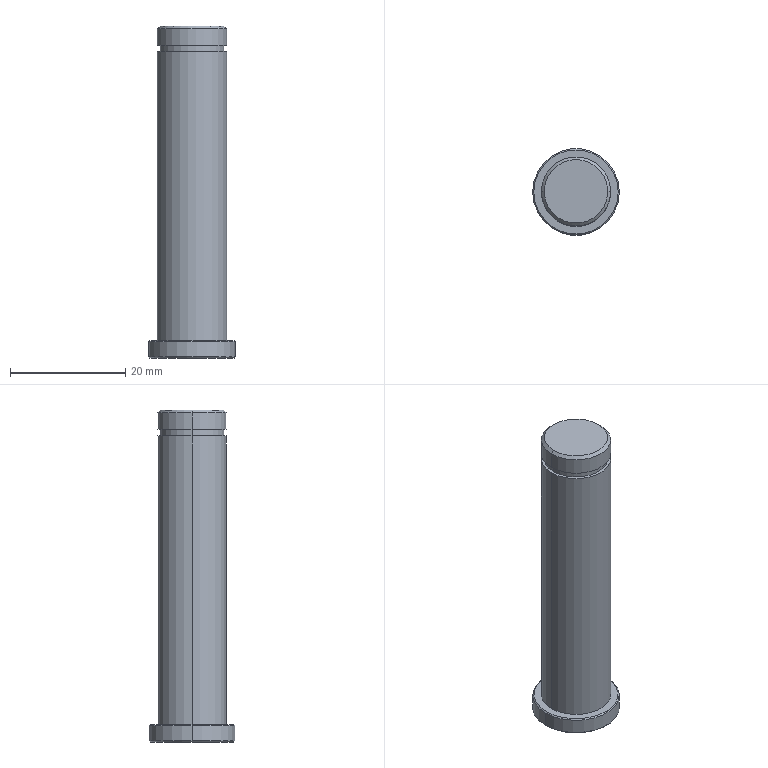Part | SolidWorks | features Chamfer 2, Extrusion 1, ICE 1, RefAxis 1, RevCut 1 | 1 solid | 19 faces | box 15 x 15 x 57.5 mm | volume 6667 mm3 | cylinder 8 | cone 6 | plane 5 | commonest cylinder face diameters 12 x4 11 x2 15 x2
STEP:
#1=CARTESIAN_POINT('',(5.5,0.,57.5));
#2=VERTEX_POINT('',#1);
#3=CARTESIAN_POINT('',(-5.5,0.,57.5));
#4=VERTEX_POINT('',#3);
#5=CARTESIAN_POINT('',(0.,0.,57.5));
#6=DIRECTION('',(0.,0.,1.));
#7=DIRECTION('',(1.,0.,0.));
#8=AXIS2_PLACEMENT_3D('',#5,#6,#7);
#9=CIRCLE('',#8,5.5);
#10=EDGE_CURVE('',#2,#4,#9,.T.);
#11=ORIENTED_EDGE('',*,*,#10,.F.);
#12=CARTESIAN_POINT('',(6.,0.,57.));
#13=VERTEX_POINT('',#12);
#14=CARTESIAN_POINT('',(5.5,0.,57.5));
#15=DIRECTION('',(0.7071,0.,-0.7071));
#16=VECTOR('',#15,1000.);
#17=LINE('',#14,#16);
#18=EDGE_CURVE('',#2,#13,#17,.T.);
#19=ORIENTED_EDGE('',*,*,#18,.T.);
#20=CARTESIAN_POINT('',(-6.,0.,57.));
#21=VERTEX_POINT('',#20);
#22=CARTESIAN_POINT('',(0.,0.,57.));
#23=DIRECTION('',(0.,0.,-1.));
#24=DIRECTION('',(1.,0.,0.));
#25=AXIS2_PLACEMENT_3D('',#22,#23,#24);
#26=CIRCLE('',#25,6.);
#27=EDGE_CURVE('',#21,#13,#26,.T.);
#28=ORIENTED_EDGE('',*,*,#27,.F.);
#29=CARTESIAN_POINT('',(-5.5,0.,57.5));
#30=DIRECTION('',(-0.7071,0.,-0.7071));
#31=VECTOR('',#30,1000.);
#32=LINE('',#29,#31);
#33=EDGE_CURVE('',#4,#21,#32,.T.);
#34=ORIENTED_EDGE('',*,*,#33,.F.);
#35=EDGE_LOOP('',(#11,#19,#28,#34));
#36=FACE_OUTER_BOUND('',#35,.T.);
#37=CARTESIAN_POINT('',(0.,0.,57.5));
#38=DIRECTION('',(0.,0.,-1.));
#39=DIRECTION('',(-1.,0.,0.));
#40=AXIS2_PLACEMENT_3D('',#37,#38,#39);
#41=CONICAL_SURFACE('',#40,5.5,0.7854);
#42=ADVANCED_FACE('',(#36),#41,.T.);
#43=ORIENTED_EDGE('',*,*,#27,.T.);
#44=CARTESIAN_POINT('',(6.,0.,54.15));
#45=VERTEX_POINT('',#44);
#46=CARTESIAN_POINT('',(6.,0.,57.5));
#47=DIRECTION('',(0.,0.,-1.));
#48=VECTOR('',#47,1000.);
#49=LINE('',#46,#48);
#50=EDGE_CURVE('',#13,#45,#49,.T.);
#51=ORIENTED_EDGE('',*,*,#50,.T.);
#52=CARTESIAN_POINT('',(-6.,0.,54.15));
#53=VERTEX_POINT('',#52);
#54=CARTESIAN_POINT('',(0.,0.,54.15));
#55=DIRECTION('',(0.,0.,1.));
#56=DIRECTION('',(1.,0.,0.));
#57=AXIS2_PLACEMENT_3D('',#54,#55,#56);
#58=CIRCLE('',#57,6.);
#59=EDGE_CURVE('',#45,#53,#58,.T.);
#60=ORIENTED_EDGE('',*,*,#59,.T.);
#61=CARTESIAN_POINT('',(-6.,0.,57.5));
#62=DIRECTION('',(0.,0.,-1.));
#63=VECTOR('',#62,1000.);
#64=LINE('',#61,#63);
#65=EDGE_CURVE('',#21,#53,#64,.T.);
#66=ORIENTED_EDGE('',*,*,#65,.F.);
#67=EDGE_LOOP('',(#43,#51,#60,#66));
#68=FACE_OUTER_BOUND('',#67,.T.);
#69=CARTESIAN_POINT('',(0.,0.,57.5));
#70=DIRECTION('',(0.,0.,-1.));
#71=DIRECTION('',(-1.,0.,0.));
#72=AXIS2_PLACEMENT_3D('',#69,#70,#71);
#73=CYLINDRICAL_SURFACE('',#72,6.);
#74=ADVANCED_FACE('',(#68),#73,.T.);
#75=CARTESIAN_POINT('',(5.5,0.,53.));
#76=VERTEX_POINT('',#75);
#77=CARTESIAN_POINT('',(-5.5,0.,53.));
#78=VERTEX_POINT('',#77);
#79=CARTESIAN_POINT('',(0.,0.,53.));
#80=DIRECTION('',(0.,0.,1.));
#81=DIRECTION('',(1.,0.,0.));
#82=AXIS2_PLACEMENT_3D('',#79,#80,#81);
#83=CIRCLE('',#82,5.5);
#84=EDGE_CURVE('',#76,#78,#83,.T.);
#85=ORIENTED_EDGE('',*,*,#84,.T.);
#86=CARTESIAN_POINT('',(-5.5,0.,54.15));
#87=VERTEX_POINT('',#86);
#88=CARTESIAN_POINT('',(-5.5,0.,57.5));
#89=DIRECTION('',(0.,0.,1.));
#90=VECTOR('',#89,1000.);
#91=LINE('',#88,#90);
#92=EDGE_CURVE('',#78,#87,#91,.T.);
#93=ORIENTED_EDGE('',*,*,#92,.T.);
#94=CARTESIAN_POINT('',(5.5,0.,54.15));
#95=VERTEX_POINT('',#94);
#96=CARTESIAN_POINT('',(0.,0.,54.15));
#97=DIRECTION('',(0.,0.,1.));
#98=DIRECTION('',(1.,0.,0.));
#99=AXIS2_PLACEMENT_3D('',#96,#97,#98);
#100=CIRCLE('',#99,5.5);
#101=EDGE_CURVE('',#95,#87,#100,.T.);
#102=ORIENTED_EDGE('',*,*,#101,.F.);
#103=CARTESIAN_POINT('',(5.5,0.,57.5));
#104=DIRECTION('',(0.,0.,1.));
#105=VECTOR('',#104,1000.);
#106=LINE('',#103,#105);
#107=EDGE_CURVE('',#76,#95,#106,.T.);
#108=ORIENTED_EDGE('',*,*,#107,.F.);
#109=EDGE_LOOP('',(#85,#93,#102,#108));
#110=FACE_OUTER_BOUND('',#109,.T.);
#111=CARTESIAN_POINT('',(0.,0.,57.5));
#112=DIRECTION('',(0.,0.,1.));
#113=DIRECTION('',(1.,0.,0.));
#114=AXIS2_PLACEMENT_3D('',#111,#112,#113);
#115=CYLINDRICAL_SURFACE('',#114,5.5);
#116=ADVANCED_FACE('',(#110),#115,.T.);
#117=CARTESIAN_POINT('',(7.3,0.,3.));
#118=VERTEX_POINT('',#117);
#119=CARTESIAN_POINT('',(-7.3,0.,3.));
#120=VERTEX_POINT('',#119);
#121=CARTESIAN_POINT('',(0.,0.,3.));
#122=DIRECTION('',(0.,0.,1.));
#123=DIRECTION('',(1.,0.,0.));
#124=AXIS2_PLACEMENT_3D('',#121,#122,#123);
#125=CIRCLE('',#124,7.3);
#126=EDGE_CURVE('',#118,#120,#125,.T.);
#127=ORIENTED_EDGE('',*,*,#126,.F.);
#128=CARTESIAN_POINT('',(7.5,0.,2.8));
#129=VERTEX_POINT('',#128);
#130=CARTESIAN_POINT('',(7.3,0.,3.));
#131=DIRECTION('',(0.7071,0.,-0.7071));
#132=VECTOR('',#131,1000.);
#133=LINE('',#130,#132);
#134=EDGE_CURVE('',#118,#129,#133,.T.);
#135=ORIENTED_EDGE('',*,*,#134,.T.);
#136=CARTESIAN_POINT('',(-7.5,0.,2.8));
#137=VERTEX_POINT('',#136);
#138=CARTESIAN_POINT('',(0.,0.,2.8));
#139=DIRECTION('',(0.,0.,-1.));
#140=DIRECTION('',(1.,0.,0.));
#141=AXIS2_PLACEMENT_3D('',#138,#139,#140);
#142=CIRCLE('',#141,7.5);
#143=EDGE_CURVE('',#137,#129,#142,.T.);
#144=ORIENTED_EDGE('',*,*,#143,.F.);
#145=CARTESIAN_POINT('',(-7.3,0.,3.));
#146=DIRECTION('',(-0.7071,0.,-0.7071));
#147=VECTOR('',#146,1000.);
#148=LINE('',#145,#147);
#149=EDGE_CURVE('',#120,#137,#148,.T.);
#150=ORIENTED_EDGE('',*,*,#149,.F.);
#151=EDGE_LOOP('',(#127,#135,#144,#150));
#152=FACE_OUTER_BOUND('',#151,.T.);
#153=CARTESIAN_POINT('',(0.,0.,3.));
#154=DIRECTION('',(0.,0.,-1.));
#155=DIRECTION('',(-1.,0.,0.));
#156=AXIS2_PLACEMENT_3D('',#153,#154,#155);
#157=CONICAL_SURFACE('',#156,7.3,0.7854);
#158=ADVANCED_FACE('',(#152),#157,.T.);
#159=CARTESIAN_POINT('',(-7.3,0.,0.));
#160=VERTEX_POINT('',#159);
#161=CARTESIAN_POINT('',(7.3,0.,0.));
#162=VERTEX_POINT('',#161);
#163=CARTESIAN_POINT('',(0.,0.,0.));
#164=DIRECTION('',(0.,0.,-1.));
#165=DIRECTION('',(1.,0.,0.));
#166=AXIS2_PLACEMENT_3D('',#163,#164,#165);
#167=CIRCLE('',#166,7.3);
#168=EDGE_CURVE('',#160,#162,#167,.T.);
#169=ORIENTED_EDGE('',*,*,#168,.F.);
#170=CARTESIAN_POINT('',(-7.5,0.,0.2));
#171=VERTEX_POINT('',#170);
#172=CARTESIAN_POINT('',(-7.5,0.,0.2));
#173=DIRECTION('',(-0.7071,0.,0.7071));
#174=VECTOR('',#173,1000.);
#175=LINE('',#172,#174);
#176=EDGE_CURVE('',#160,#171,#175,.T.);
#177=ORIENTED_EDGE('',*,*,#176,.T.);
#178=CARTESIAN_POINT('',(7.5,0.,0.2));
#179=VERTEX_POINT('',#178);
#180=CARTESIAN_POINT('',(0.,0.,0.2));
#181=DIRECTION('',(0.,0.,1.));
#182=DIRECTION('',(1.,0.,0.));
#183=AXIS2_PLACEMENT_3D('',#180,#181,#182);
#184=CIRCLE('',#183,7.5);
#185=EDGE_CURVE('',#179,#171,#184,.T.);
#186=ORIENTED_EDGE('',*,*,#185,.F.);
#187=CARTESIAN_POINT('',(7.5,0.,0.2));
#188=DIRECTION('',(0.7071,0.,0.7071));
#189=VECTOR('',#188,1000.);
#190=LINE('',#187,#189);
#191=EDGE_CURVE('',#162,#179,#190,.T.);
#192=ORIENTED_EDGE('',*,*,#191,.F.);
#193=EDGE_LOOP('',(#169,#177,#186,#192));
#194=FACE_OUTER_BOUND('',#193,.T.);
#195=CARTESIAN_POINT('',(0.,0.,0.2));
#196=DIRECTION('',(0.,0.,1.));
#197=DIRECTION('',(1.,0.,0.));
#198=AXIS2_PLACEMENT_3D('',#195,#196,#197);
#199=CONICAL_SURFACE('',#198,7.5,0.7854);
#200=ADVANCED_FACE('',(#194),#199,.T.);
#201=ORIENTED_EDGE('',*,*,#143,.T.);
#202=CARTESIAN_POINT('',(7.5,0.,3.));
#203=DIRECTION('',(0.,0.,-1.));
#204=VECTOR('',#203,1000.);
#205=LINE('',#202,#204);
#206=EDGE_CURVE('',#129,#179,#205,.T.);
#207=ORIENTED_EDGE('',*,*,#206,.T.);
#208=ORIENTED_EDGE('',*,*,#185,.T.);
#209=CARTESIAN_POINT('',(-7.5,0.,3.));
#210=DIRECTION('',(0.,0.,-1.));
#211=VECTOR('',#210,1000.);
#212=LINE('',#209,#211);
#213=EDGE_CURVE('',#137,#171,#212,.T.);
#214=ORIENTED_EDGE('',*,*,#213,.F.);
#215=EDGE_LOOP('',(#201,#207,#208,#214));
#216=FACE_OUTER_BOUND('',#215,.T.);
#217=CARTESIAN_POINT('',(0.,0.,3.));
#218=DIRECTION('',(0.,0.,-1.));
#219=DIRECTION('',(-1.,0.,0.));
#220=AXIS2_PLACEMENT_3D('',#217,#218,#219);
#221=CYLINDRICAL_SURFACE('',#220,7.5);
#222=ADVANCED_FACE('',(#216),#221,.T.);
#223=CARTESIAN_POINT('',(6.,0.,53.));
#224=VERTEX_POINT('',#223);
#225=CARTESIAN_POINT('',(-6.,0.,53.));
#226=VERTEX_POINT('',#225);
#227=CARTESIAN_POINT('',(0.,0.,53.));
#228=DIRECTION('',(0.,0.,1.));
#229=DIRECTION('',(1.,0.,0.));
#230=AXIS2_PLACEMENT_3D('',#227,#228,#229);
#231=CIRCLE('',#230,6.);
#232=EDGE_CURVE('',#224,#226,#231,.T.);
#233=ORIENTED_EDGE('',*,*,#232,.F.);
#234=CARTESIAN_POINT('',(6.,0.,3.));
#235=VERTEX_POINT('',#234);
#236=CARTESIAN_POINT('',(6.,0.,57.5));
#237=DIRECTION('',(0.,0.,-1.));
#238=VECTOR('',#237,1000.);
#239=LINE('',#236,#238);
#240=EDGE_CURVE('',#224,#235,#239,.T.);
#241=ORIENTED_EDGE('',*,*,#240,.T.);
#242=CARTESIAN_POINT('',(-6.,0.,3.));
#243=VERTEX_POINT('',#242);
#244=CARTESIAN_POINT('',(0.,0.,3.));
#245=DIRECTION('',(0.,0.,1.));
#246=DIRECTION('',(1.,0.,0.));
#247=AXIS2_PLACEMENT_3D('',#244,#245,#246);
#248=CIRCLE('',#247,6.);
#249=EDGE_CURVE('',#235,#243,#248,.T.);
#250=ORIENTED_EDGE('',*,*,#249,.T.);
#251=CARTESIAN_POINT('',(-6.,0.,57.5));
#252=DIRECTION('',(0.,0.,-1.));
#253=VECTOR('',#252,1000.);
#254=LINE('',#251,#253);
#255=EDGE_CURVE('',#226,#243,#254,.T.);
#256=ORIENTED_EDGE('',*,*,#255,.F.);
#257=EDGE_LOOP('',(#233,#241,#250,#256));
#258=FACE_OUTER_BOUND('',#257,.T.);
#259=CARTESIAN_POINT('',(0.,0.,57.5));
#260=DIRECTION('',(0.,0.,-1.));
#261=DIRECTION('',(-1.,0.,0.));
#262=AXIS2_PLACEMENT_3D('',#259,#260,#261);
#263=CYLINDRICAL_SURFACE('',#262,6.);
#264=ADVANCED_FACE('',(#258),#263,.T.);
#265=ORIENTED_EDGE('',*,*,#240,.F.);
#266=CARTESIAN_POINT('',(0.,0.,53.));
#267=DIRECTION('',(0.,0.,1.));
#268=DIRECTION('',(1.,0.,0.));
#269=AXIS2_PLACEMENT_3D('',#266,#267,#268);
#270=CIRCLE('',#269,6.);
#271=EDGE_CURVE('',#226,#224,#270,.T.);
#272=ORIENTED_EDGE('',*,*,#271,.F.);
#273=ORIENTED_EDGE('',*,*,#255,.T.);
#274=CARTESIAN_POINT('',(0.,0.,3.));
#275=DIRECTION('',(0.,0.,1.));
#276=DIRECTION('',(1.,0.,0.));
#277=AXIS2_PLACEMENT_3D('',#274,#275,#276);
#278=CIRCLE('',#277,6.);
#279=EDGE_CURVE('',#243,#235,#278,.T.);
#280=ORIENTED_EDGE('',*,*,#279,.T.);
#281=EDGE_LOOP('',(#265,#272,#273,#280));
#282=FACE_OUTER_BOUND('',#281,.T.);
#283=CARTESIAN_POINT('',(0.,0.,57.5));
#284=DIRECTION('',(0.,0.,-1.));
#285=DIRECTION('',(-1.,0.,0.));
#286=AXIS2_PLACEMENT_3D('',#283,#284,#285);
#287=CYLINDRICAL_SURFACE('',#286,6.);
#288=ADVANCED_FACE('',(#282),#287,.T.);
#289=CARTESIAN_POINT('',(0.,0.,3.));
#290=DIRECTION('',(0.,0.,1.));
#291=DIRECTION('',(1.,0.,0.));
#292=AXIS2_PLACEMENT_3D('',#289,#290,#291);
#293=CIRCLE('',#292,7.3);
#294=EDGE_CURVE('',#120,#118,#293,.T.);
#295=ORIENTED_EDGE('',*,*,#294,.T.);
#296=ORIENTED_EDGE('',*,*,#126,.T.);
#297=EDGE_LOOP('',(#295,#296));
#298=FACE_OUTER_BOUND('',#297,.T.);
#299=ORIENTED_EDGE('',*,*,#279,.F.);
#300=ORIENTED_EDGE('',*,*,#249,.F.);
#301=EDGE_LOOP('',(#299,#300));
#302=FACE_BOUND('',#301,.T.);
#303=CARTESIAN_POINT('',(0.,0.,3.));
#304=DIRECTION('',(0.,0.,1.));
#305=DIRECTION('',(1.,0.,0.));
#306=AXIS2_PLACEMENT_3D('',#303,#304,#305);
#307=PLANE('',#306);
#308=ADVANCED_FACE('',(#298,#302),#307,.T.);
#309=ORIENTED_EDGE('',*,*,#206,.F.);
#310=CARTESIAN_POINT('',(0.,0.,2.8));
#311=DIRECTION('',(0.,0.,-1.));
#312=DIRECTION('',(1.,0.,0.));
#313=AXIS2_PLACEMENT_3D('',#310,#311,#312);
#314=CIRCLE('',#313,7.5);
#315=EDGE_CURVE('',#129,#137,#314,.T.);
#316=ORIENTED_EDGE('',*,*,#315,.T.);
#317=ORIENTED_EDGE('',*,*,#213,.T.);
#318=CARTESIAN_POINT('',(0.,0.,0.2));
#319=DIRECTION('',(0.,0.,1.));
#320=DIRECTION('',(1.,0.,0.));
#321=AXIS2_PLACEMENT_3D('',#318,#319,#320);
#322=CIRCLE('',#321,7.5);
#323=EDGE_CURVE('',#171,#179,#322,.T.);
#324=ORIENTED_EDGE('',*,*,#323,.T.);
#325=EDGE_LOOP('',(#309,#316,#317,#324));
#326=FACE_OUTER_BOUND('',#325,.T.);
#327=CARTESIAN_POINT('',(0.,0.,3.));
#328=DIRECTION('',(0.,0.,-1.));
#329=DIRECTION('',(-1.,0.,0.));
#330=AXIS2_PLACEMENT_3D('',#327,#328,#329);
#331=CYLINDRICAL_SURFACE('',#330,7.5);
#332=ADVANCED_FACE('',(#326),#331,.T.);
#333=CARTESIAN_POINT('',(0.,0.,0.));
#334=DIRECTION('',(0.,0.,-1.));
#335=DIRECTION('',(1.,0.,0.));
#336=AXIS2_PLACEMENT_3D('',#333,#334,#335);
#337=CIRCLE('',#336,7.3);
#338=EDGE_CURVE('',#162,#160,#337,.T.);
#339=ORIENTED_EDGE('',*,*,#338,.T.);
#340=ORIENTED_EDGE('',*,*,#168,.T.);
#341=EDGE_LOOP('',(#339,#340));
#342=FACE_OUTER_BOUND('',#341,.T.);
#343=CARTESIAN_POINT('',(0.,0.,0.));
#344=DIRECTION('',(0.,0.,1.));
#345=DIRECTION('',(1.,0.,0.));
#346=AXIS2_PLACEMENT_3D('',#343,#344,#345);
#347=PLANE('',#346);
#348=ADVANCED_FACE('',(#342),#347,.F.);
#349=ORIENTED_EDGE('',*,*,#176,.F.);
#350=ORIENTED_EDGE('',*,*,#338,.F.);
#351=ORIENTED_EDGE('',*,*,#191,.T.);
#352=ORIENTED_EDGE('',*,*,#323,.F.);
#353=EDGE_LOOP('',(#349,#350,#351,#352));
#354=FACE_OUTER_BOUND('',#353,.T.);
#355=CARTESIAN_POINT('',(0.,0.,0.2));
#356=DIRECTION('',(0.,0.,1.));
#357=DIRECTION('',(1.,0.,0.));
#358=AXIS2_PLACEMENT_3D('',#355,#356,#357);
#359=CONICAL_SURFACE('',#358,7.5,0.7854);
#360=ADVANCED_FACE('',(#354),#359,.T.);
#361=ORIENTED_EDGE('',*,*,#134,.F.);
#362=ORIENTED_EDGE('',*,*,#294,.F.);
#363=ORIENTED_EDGE('',*,*,#149,.T.);
#364=ORIENTED_EDGE('',*,*,#315,.F.);
#365=EDGE_LOOP('',(#361,#362,#363,#364));
#366=FACE_OUTER_BOUND('',#365,.T.);
#367=CARTESIAN_POINT('',(0.,0.,3.));
#368=DIRECTION('',(0.,0.,-1.));
#369=DIRECTION('',(-1.,0.,0.));
#370=AXIS2_PLACEMENT_3D('',#367,#368,#369);
#371=CONICAL_SURFACE('',#370,7.3,0.7854);
#372=ADVANCED_FACE('',(#366),#371,.T.);
#373=ORIENTED_EDGE('',*,*,#271,.T.);
#374=ORIENTED_EDGE('',*,*,#232,.T.);
#375=EDGE_LOOP('',(#373,#374));
#376=FACE_OUTER_BOUND('',#375,.T.);
#377=ORIENTED_EDGE('',*,*,#84,.F.);
#378=CARTESIAN_POINT('',(0.,0.,53.));
#379=DIRECTION('',(0.,0.,1.));
#380=DIRECTION('',(1.,0.,0.));
#381=AXIS2_PLACEMENT_3D('',#378,#379,#380);
#382=CIRCLE('',#381,5.5);
#383=EDGE_CURVE('',#78,#76,#382,.T.);
#384=ORIENTED_EDGE('',*,*,#383,.F.);
#385=EDGE_LOOP('',(#377,#384));
#386=FACE_BOUND('',#385,.T.);
#387=CARTESIAN_POINT('',(-6.,0.,53.));
#388=DIRECTION('',(0.,0.,1.));
#389=DIRECTION('',(1.,0.,0.));
#390=AXIS2_PLACEMENT_3D('',#387,#388,#389);
#391=PLANE('',#390);
#392=ADVANCED_FACE('',(#376,#386),#391,.T.);
#393=ORIENTED_EDGE('',*,*,#92,.F.);
#394=ORIENTED_EDGE('',*,*,#383,.T.);
#395=ORIENTED_EDGE('',*,*,#107,.T.);
#396=CARTESIAN_POINT('',(0.,0.,54.15));
#397=DIRECTION('',(0.,0.,1.));
#398=DIRECTION('',(1.,0.,0.));
#399=AXIS2_PLACEMENT_3D('',#396,#397,#398);
#400=CIRCLE('',#399,5.5);
#401=EDGE_CURVE('',#87,#95,#400,.T.);
#402=ORIENTED_EDGE('',*,*,#401,.F.);
#403=EDGE_LOOP('',(#393,#394,#395,#402));
#404=FACE_OUTER_BOUND('',#403,.T.);
#405=CARTESIAN_POINT('',(0.,0.,57.5));
#406=DIRECTION('',(0.,0.,1.));
#407=DIRECTION('',(1.,0.,0.));
#408=AXIS2_PLACEMENT_3D('',#405,#406,#407);
#409=CYLINDRICAL_SURFACE('',#408,5.5);
#410=ADVANCED_FACE('',(#404),#409,.T.);
#411=ORIENTED_EDGE('',*,*,#101,.T.);
#412=ORIENTED_EDGE('',*,*,#401,.T.);
#413=EDGE_LOOP('',(#411,#412));
#414=FACE_BOUND('',#413,.T.);
#415=CARTESIAN_POINT('',(0.,0.,54.15));
#416=DIRECTION('',(0.,0.,1.));
#417=DIRECTION('',(1.,0.,0.));
#418=AXIS2_PLACEMENT_3D('',#415,#416,#417);
#419=CIRCLE('',#418,6.);
#420=EDGE_CURVE('',#53,#45,#419,.T.);
#421=ORIENTED_EDGE('',*,*,#420,.F.);
#422=ORIENTED_EDGE('',*,*,#59,.F.);
#423=EDGE_LOOP('',(#421,#422));
#424=FACE_OUTER_BOUND('',#423,.T.);
#425=CARTESIAN_POINT('',(-6.,0.,54.15));
#426=DIRECTION('',(0.,0.,-1.));
#427=DIRECTION('',(-1.,0.,0.));
#428=AXIS2_PLACEMENT_3D('',#425,#426,#427);
#429=PLANE('',#428);
#430=ADVANCED_FACE('',(#414,#424),#429,.T.);
#431=CARTESIAN_POINT('',(0.,0.,57.5));
#432=DIRECTION('',(0.,0.,1.));
#433=DIRECTION('',(1.,0.,0.));
#434=AXIS2_PLACEMENT_3D('',#431,#432,#433);
#435=CIRCLE('',#434,5.5);
#436=EDGE_CURVE('',#4,#2,#435,.T.);
#437=ORIENTED_EDGE('',*,*,#436,.T.);
#438=ORIENTED_EDGE('',*,*,#10,.T.);
#439=EDGE_LOOP('',(#437,#438));
#440=FACE_OUTER_BOUND('',#439,.T.);
#441=CARTESIAN_POINT('',(0.,0.,57.5));
#442=DIRECTION('',(0.,0.,1.));
#443=DIRECTION('',(1.,0.,0.));
#444=AXIS2_PLACEMENT_3D('',#441,#442,#443);
#445=PLANE('',#444);
#446=ADVANCED_FACE('',(#440),#445,.T.);
#447=ORIENTED_EDGE('',*,*,#50,.F.);
#448=CARTESIAN_POINT('',(0.,0.,57.));
#449=DIRECTION('',(0.,0.,-1.));
#450=DIRECTION('',(1.,0.,0.));
#451=AXIS2_PLACEMENT_3D('',#448,#449,#450);
#452=CIRCLE('',#451,6.);
#453=EDGE_CURVE('',#13,#21,#452,.T.);
#454=ORIENTED_EDGE('',*,*,#453,.T.);
#455=ORIENTED_EDGE('',*,*,#65,.T.);
#456=ORIENTED_EDGE('',*,*,#420,.T.);
#457=EDGE_LOOP('',(#447,#454,#455,#456));
#458=FACE_OUTER_BOUND('',#457,.T.);
#459=CARTESIAN_POINT('',(0.,0.,57.5));
#460=DIRECTION('',(0.,0.,-1.));
#461=DIRECTION('',(-1.,0.,0.));
#462=AXIS2_PLACEMENT_3D('',#459,#460,#461);
#463=CYLINDRICAL_SURFACE('',#462,6.);
#464=ADVANCED_FACE('',(#458),#463,.T.);
#465=ORIENTED_EDGE('',*,*,#18,.F.);
#466=ORIENTED_EDGE('',*,*,#436,.F.);
#467=ORIENTED_EDGE('',*,*,#33,.T.);
#468=ORIENTED_EDGE('',*,*,#453,.F.);
#469=EDGE_LOOP('',(#465,#466,#467,#468));
#470=FACE_OUTER_BOUND('',#469,.T.);
#471=CARTESIAN_POINT('',(0.,0.,57.5));
#472=DIRECTION('',(0.,0.,-1.));
#473=DIRECTION('',(-1.,0.,0.));
#474=AXIS2_PLACEMENT_3D('',#471,#472,#473);
#475=CONICAL_SURFACE('',#474,5.5,0.7854);
#476=ADVANCED_FACE('',(#470),#475,.T.);
#477=CLOSED_SHELL('',(#42,#74,#116,#158,#200,#222,#264,#288,#308,#332,#348,#360,#372,#392,#410,#430,#446,#464,#476));
#478=MANIFOLD_SOLID_BREP('',#477);
#479=CARTESIAN_POINT('',(0.,0.,0.));
#480=DIRECTION('',(0.,0.,1.));
#481=DIRECTION('',(1.,0.,0.));
#482=AXIS2_PLACEMENT_3D('',#479,#480,#481);
#483=(LENGTH_UNIT()NAMED_UNIT(*)SI_UNIT(.MILLI.,.METRE.));
#484=UNCERTAINTY_MEASURE_WITH_UNIT(LENGTH_MEASURE(0.00001),#483,'','');
#485=(NAMED_UNIT(*)PLANE_ANGLE_UNIT()SI_UNIT($,.RADIAN.));
#486=(NAMED_UNIT(*)SI_UNIT($,.STERADIAN.)SOLID_ANGLE_UNIT());
#487=(GEOMETRIC_REPRESENTATION_CONTEXT(3)GLOBAL_UNCERTAINTY_ASSIGNED_CONTEXT((#484))GLOBAL_UNIT_ASSIGNED_CONTEXT((#483,#485,#486))REPRESENTATION_CONTEXT('',''));
#488=ADVANCED_BREP_SHAPE_REPRESENTATION('',(#478,#482),#487);